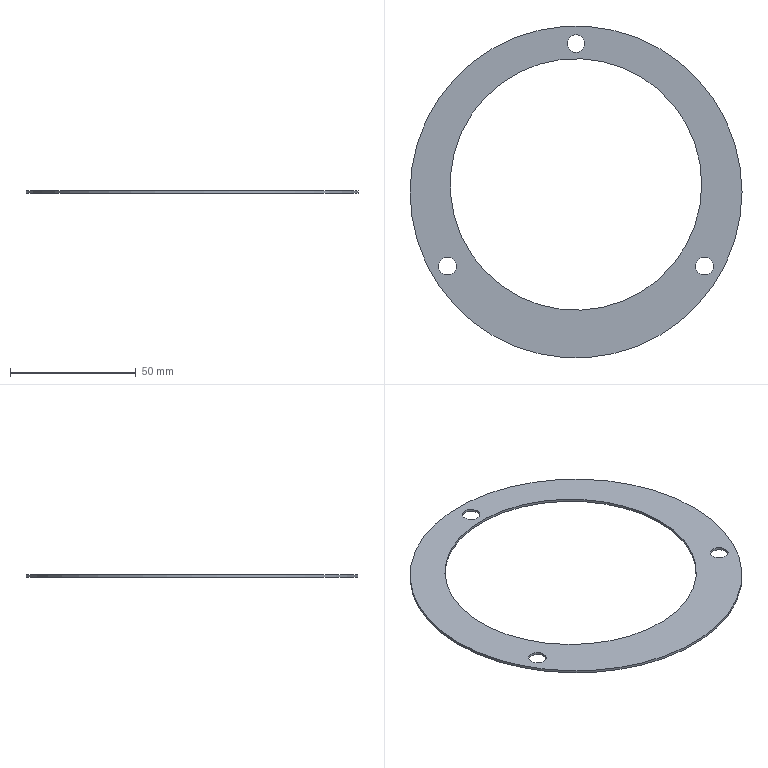Part | NX | features DATUM_CSYS 2, EXTRUDE 1, SKETCH 1 | 1 solid | 7 faces | box 132 x 132 x 1 mm | volume 5715 mm3 | cylinder 5 | plane 2 | commonest cylinder face diameters 7 x3 100 x1 132 x1
STEP:
#1=CARTESIAN_POINT('',(50.,0.,1.));
#2=VERTEX_POINT('',#1);
#3=CARTESIAN_POINT('',(0.,0.,1.));
#4=DIRECTION('',(0.,0.,1.));
#5=DIRECTION('',(1.,0.,0.));
#6=AXIS2_PLACEMENT_3D('',#3,#4,#5);
#7=CIRCLE('',#6,50.);
#8=EDGE_CURVE('',#2,#2,#7,.T.);
#9=ORIENTED_EDGE('',*,*,#8,.T.);
#10=EDGE_LOOP('',(#9));
#11=FACE_BOUND('',#10,.T.);
#12=CARTESIAN_POINT('',(50.,0.,0.));
#13=VERTEX_POINT('',#12);
#14=CARTESIAN_POINT('',(0.,0.,0.));
#15=DIRECTION('',(0.,0.,1.));
#16=DIRECTION('',(1.,0.,0.));
#17=AXIS2_PLACEMENT_3D('',#14,#15,#16);
#18=CIRCLE('',#17,50.);
#19=EDGE_CURVE('',#13,#13,#18,.T.);
#20=ORIENTED_EDGE('',*,*,#19,.F.);
#21=EDGE_LOOP('',(#20));
#22=FACE_BOUND('',#21,.T.);
#23=CARTESIAN_POINT('',(0.,0.,1.));
#24=DIRECTION('',(0.,0.,-1.));
#25=DIRECTION('',(-1.,0.,0.));
#26=AXIS2_PLACEMENT_3D('',#23,#24,#25);
#27=CYLINDRICAL_SURFACE('',#26,50.);
#28=ADVANCED_FACE('',(#11,#22),#27,.F.);
#29=CARTESIAN_POINT('',(3.5,56.,1.));
#30=VERTEX_POINT('',#29);
#31=CARTESIAN_POINT('',(0.,56.,1.));
#32=DIRECTION('',(0.,0.,1.));
#33=DIRECTION('',(1.,0.,0.));
#34=AXIS2_PLACEMENT_3D('',#31,#32,#33);
#35=CIRCLE('',#34,3.5);
#36=EDGE_CURVE('',#30,#30,#35,.T.);
#37=ORIENTED_EDGE('',*,*,#36,.T.);
#38=EDGE_LOOP('',(#37));
#39=FACE_BOUND('',#38,.T.);
#40=CARTESIAN_POINT('',(3.5,56.,0.));
#41=VERTEX_POINT('',#40);
#42=CARTESIAN_POINT('',(0.,56.,0.));
#43=DIRECTION('',(0.,0.,1.));
#44=DIRECTION('',(1.,0.,0.));
#45=AXIS2_PLACEMENT_3D('',#42,#43,#44);
#46=CIRCLE('',#45,3.5);
#47=EDGE_CURVE('',#41,#41,#46,.T.);
#48=ORIENTED_EDGE('',*,*,#47,.F.);
#49=EDGE_LOOP('',(#48));
#50=FACE_BOUND('',#49,.T.);
#51=CARTESIAN_POINT('',(0.,56.,1.));
#52=DIRECTION('',(0.,0.,-1.));
#53=DIRECTION('',(-1.,0.,0.));
#54=AXIS2_PLACEMENT_3D('',#51,#52,#53);
#55=CYLINDRICAL_SURFACE('',#54,3.5);
#56=ADVANCED_FACE('',(#39,#50),#55,.F.);
#57=CARTESIAN_POINT('',(54.595,-32.5,1.));
#58=VERTEX_POINT('',#57);
#59=CARTESIAN_POINT('',(51.095,-32.5,1.));
#60=DIRECTION('',(0.,0.,1.));
#61=DIRECTION('',(1.,0.,0.));
#62=AXIS2_PLACEMENT_3D('',#59,#60,#61);
#63=CIRCLE('',#62,3.5);
#64=EDGE_CURVE('',#58,#58,#63,.T.);
#65=ORIENTED_EDGE('',*,*,#64,.T.);
#66=EDGE_LOOP('',(#65));
#67=FACE_BOUND('',#66,.T.);
#68=CARTESIAN_POINT('',(54.595,-32.5,0.));
#69=VERTEX_POINT('',#68);
#70=CARTESIAN_POINT('',(51.095,-32.5,0.));
#71=DIRECTION('',(0.,0.,1.));
#72=DIRECTION('',(1.,0.,0.));
#73=AXIS2_PLACEMENT_3D('',#70,#71,#72);
#74=CIRCLE('',#73,3.5);
#75=EDGE_CURVE('',#69,#69,#74,.T.);
#76=ORIENTED_EDGE('',*,*,#75,.F.);
#77=EDGE_LOOP('',(#76));
#78=FACE_BOUND('',#77,.T.);
#79=CARTESIAN_POINT('',(51.095,-32.5,1.));
#80=DIRECTION('',(0.,0.,-1.));
#81=DIRECTION('',(-1.,0.,0.));
#82=AXIS2_PLACEMENT_3D('',#79,#80,#81);
#83=CYLINDRICAL_SURFACE('',#82,3.5);
#84=ADVANCED_FACE('',(#67,#78),#83,.F.);
#85=CARTESIAN_POINT('',(66.,-3.,1.));
#86=VERTEX_POINT('',#85);
#87=CARTESIAN_POINT('',(0.,-3.,1.));
#88=DIRECTION('',(0.,0.,1.));
#89=DIRECTION('',(1.,0.,0.));
#90=AXIS2_PLACEMENT_3D('',#87,#88,#89);
#91=CIRCLE('',#90,66.);
#92=EDGE_CURVE('',#86,#86,#91,.T.);
#93=ORIENTED_EDGE('',*,*,#92,.F.);
#94=EDGE_LOOP('',(#93));
#95=FACE_BOUND('',#94,.T.);
#96=CARTESIAN_POINT('',(66.,-3.,0.));
#97=VERTEX_POINT('',#96);
#98=CARTESIAN_POINT('',(0.,-3.,0.));
#99=DIRECTION('',(0.,0.,1.));
#100=DIRECTION('',(1.,0.,0.));
#101=AXIS2_PLACEMENT_3D('',#98,#99,#100);
#102=CIRCLE('',#101,66.);
#103=EDGE_CURVE('',#97,#97,#102,.T.);
#104=ORIENTED_EDGE('',*,*,#103,.T.);
#105=EDGE_LOOP('',(#104));
#106=FACE_BOUND('',#105,.T.);
#107=CARTESIAN_POINT('',(0.,-3.,1.));
#108=DIRECTION('',(0.,0.,-1.));
#109=DIRECTION('',(-1.,0.,0.));
#110=AXIS2_PLACEMENT_3D('',#107,#108,#109);
#111=CYLINDRICAL_SURFACE('',#110,66.);
#112=ADVANCED_FACE('',(#95,#106),#111,.T.);
#113=CARTESIAN_POINT('',(-47.595,-32.5,1.));
#114=VERTEX_POINT('',#113);
#115=CARTESIAN_POINT('',(-51.095,-32.5,1.));
#116=DIRECTION('',(0.,0.,1.));
#117=DIRECTION('',(1.,0.,0.));
#118=AXIS2_PLACEMENT_3D('',#115,#116,#117);
#119=CIRCLE('',#118,3.5);
#120=EDGE_CURVE('',#114,#114,#119,.T.);
#121=ORIENTED_EDGE('',*,*,#120,.T.);
#122=EDGE_LOOP('',(#121));
#123=FACE_BOUND('',#122,.T.);
#124=CARTESIAN_POINT('',(-47.595,-32.5,0.));
#125=VERTEX_POINT('',#124);
#126=CARTESIAN_POINT('',(-51.095,-32.5,0.));
#127=DIRECTION('',(0.,0.,1.));
#128=DIRECTION('',(1.,0.,0.));
#129=AXIS2_PLACEMENT_3D('',#126,#127,#128);
#130=CIRCLE('',#129,3.5);
#131=EDGE_CURVE('',#125,#125,#130,.T.);
#132=ORIENTED_EDGE('',*,*,#131,.F.);
#133=EDGE_LOOP('',(#132));
#134=FACE_BOUND('',#133,.T.);
#135=CARTESIAN_POINT('',(-51.095,-32.5,1.));
#136=DIRECTION('',(0.,0.,-1.));
#137=DIRECTION('',(-1.,0.,0.));
#138=AXIS2_PLACEMENT_3D('',#135,#136,#137);
#139=CYLINDRICAL_SURFACE('',#138,3.5);
#140=ADVANCED_FACE('',(#123,#134),#139,.F.);
#141=ORIENTED_EDGE('',*,*,#92,.T.);
#142=EDGE_LOOP('',(#141));
#143=FACE_BOUND('',#142,.T.);
#144=ORIENTED_EDGE('',*,*,#64,.F.);
#145=EDGE_LOOP('',(#144));
#146=FACE_BOUND('',#145,.T.);
#147=ORIENTED_EDGE('',*,*,#36,.F.);
#148=EDGE_LOOP('',(#147));
#149=FACE_BOUND('',#148,.T.);
#150=ORIENTED_EDGE('',*,*,#8,.F.);
#151=EDGE_LOOP('',(#150));
#152=FACE_BOUND('',#151,.T.);
#153=ORIENTED_EDGE('',*,*,#120,.F.);
#154=EDGE_LOOP('',(#153));
#155=FACE_BOUND('',#154,.T.);
#156=CARTESIAN_POINT('',(25.548,-17.75,1.));
#157=DIRECTION('',(0.,0.,1.));
#158=DIRECTION('',(1.,0.,0.));
#159=AXIS2_PLACEMENT_3D('',#156,#157,#158);
#160=PLANE('',#159);
#161=ADVANCED_FACE('',(#143,#146,#149,#152,#155),#160,.T.);
#162=ORIENTED_EDGE('',*,*,#103,.F.);
#163=EDGE_LOOP('',(#162));
#164=FACE_BOUND('',#163,.T.);
#165=ORIENTED_EDGE('',*,*,#75,.T.);
#166=EDGE_LOOP('',(#165));
#167=FACE_BOUND('',#166,.T.);
#168=ORIENTED_EDGE('',*,*,#47,.T.);
#169=EDGE_LOOP('',(#168));
#170=FACE_BOUND('',#169,.T.);
#171=ORIENTED_EDGE('',*,*,#19,.T.);
#172=EDGE_LOOP('',(#171));
#173=FACE_BOUND('',#172,.T.);
#174=ORIENTED_EDGE('',*,*,#131,.T.);
#175=EDGE_LOOP('',(#174));
#176=FACE_BOUND('',#175,.T.);
#177=CARTESIAN_POINT('',(25.548,-17.75,0.));
#178=DIRECTION('',(0.,0.,1.));
#179=DIRECTION('',(1.,0.,0.));
#180=AXIS2_PLACEMENT_3D('',#177,#178,#179);
#181=PLANE('',#180);
#182=ADVANCED_FACE('',(#164,#167,#170,#173,#176),#181,.F.);
#183=CLOSED_SHELL('',(#28,#56,#84,#112,#140,#161,#182));
#184=MANIFOLD_SOLID_BREP('',#183);
#185=(LENGTH_UNIT()NAMED_UNIT(*)SI_UNIT(.MILLI.,.METRE.));
#186=UNCERTAINTY_MEASURE_WITH_UNIT(LENGTH_MEASURE(0.00001),#185,'','');
#187=(NAMED_UNIT(*)PLANE_ANGLE_UNIT()SI_UNIT($,.RADIAN.));
#188=(NAMED_UNIT(*)SI_UNIT($,.STERADIAN.)SOLID_ANGLE_UNIT());
#189=(GEOMETRIC_REPRESENTATION_CONTEXT(3)GLOBAL_UNCERTAINTY_ASSIGNED_CONTEXT((#186))GLOBAL_UNIT_ASSIGNED_CONTEXT((#185,#187,#188))REPRESENTATION_CONTEXT('',''));
#190=ADVANCED_BREP_SHAPE_REPRESENTATION('',(#184),#189);